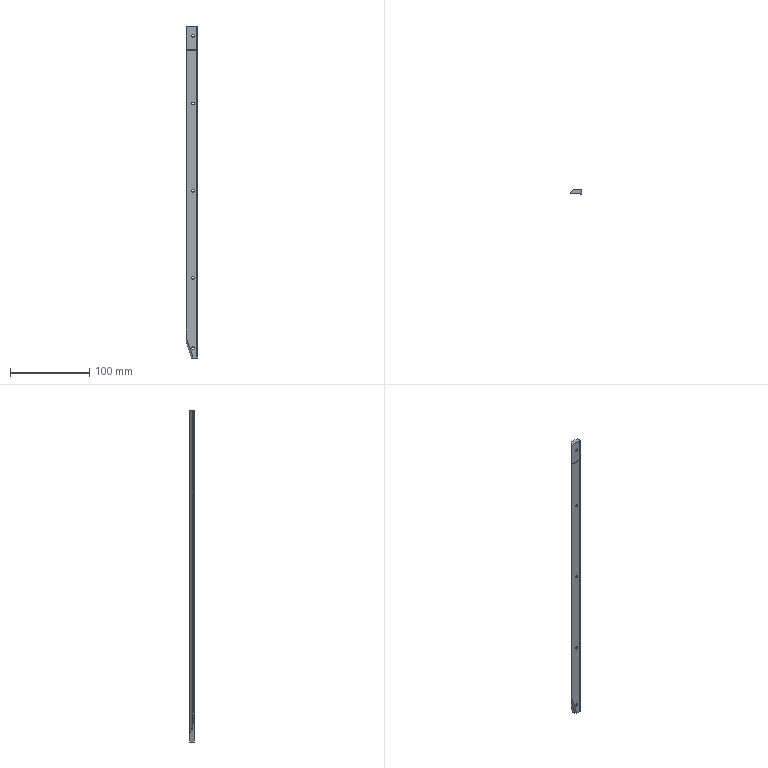Part | STEP file | 11-FG-B07511 | 1 solid | 43 faces | box 14.5 x 6 x 419 mm | volume 26571 mm3 | plane 22 | cylinder 21 | commonest cylinder face diameters 3.4 x10 6.5 x10 0.85 x1
STEP:
#1=CARTESIAN_POINT('',(8.5,1.6,403.25));
#2=VERTEX_POINT('',#1);
#3=CARTESIAN_POINT('',(8.5,1.6,409.75));
#4=VERTEX_POINT('',#3);
#5=CARTESIAN_POINT('',(8.5,1.6,406.5));
#6=DIRECTION('',(0.,1.,0.));
#7=DIRECTION('',(0.,0.,1.));
#8=AXIS2_PLACEMENT_3D('',#5,#6,#7);
#9=CIRCLE('',#8,3.25);
#10=EDGE_CURVE('',#2,#4,#9,.T.);
#11=ORIENTED_EDGE('',*,*,#10,.F.);
#12=CARTESIAN_POINT('',(8.5,5.,403.25));
#13=VERTEX_POINT('',#12);
#14=CARTESIAN_POINT('',(8.5,5.,403.25));
#15=DIRECTION('',(0.,1.,0.));
#16=VECTOR('',#15,1000.);
#17=LINE('',#14,#16);
#18=EDGE_CURVE('',#2,#13,#17,.T.);
#19=ORIENTED_EDGE('',*,*,#18,.T.);
#20=CARTESIAN_POINT('',(8.5,5.,409.75));
#21=VERTEX_POINT('',#20);
#22=CARTESIAN_POINT('',(8.5,5.,406.5));
#23=DIRECTION('',(0.,1.,0.));
#24=DIRECTION('',(0.,0.,1.));
#25=AXIS2_PLACEMENT_3D('',#22,#23,#24);
#26=CIRCLE('',#25,3.25);
#27=EDGE_CURVE('',#13,#21,#26,.T.);
#28=ORIENTED_EDGE('',*,*,#27,.T.);
#29=CARTESIAN_POINT('',(8.5,5.,409.75));
#30=DIRECTION('',(0.,1.,0.));
#31=VECTOR('',#30,1000.);
#32=LINE('',#29,#31);
#33=EDGE_CURVE('',#4,#21,#32,.T.);
#34=ORIENTED_EDGE('',*,*,#33,.F.);
#35=EDGE_LOOP('',(#11,#19,#28,#34));
#36=FACE_OUTER_BOUND('',#35,.T.);
#37=CARTESIAN_POINT('',(8.5,5.,406.5));
#38=DIRECTION('',(0.,1.,0.));
#39=DIRECTION('',(0.,0.,1.));
#40=AXIS2_PLACEMENT_3D('',#37,#38,#39);
#41=CYLINDRICAL_SURFACE('',#40,3.25);
#42=ADVANCED_FACE('',(#36),#41,.F.);
#43=CARTESIAN_POINT('',(8.5,0.,404.8));
#44=VERTEX_POINT('',#43);
#45=CARTESIAN_POINT('',(8.5,0.,408.2));
#46=VERTEX_POINT('',#45);
#47=CARTESIAN_POINT('',(8.5,0.,406.5));
#48=DIRECTION('',(0.,1.,0.));
#49=DIRECTION('',(0.,0.,1.));
#50=AXIS2_PLACEMENT_3D('',#47,#48,#49);
#51=CIRCLE('',#50,1.7);
#52=EDGE_CURVE('',#44,#46,#51,.T.);
#53=ORIENTED_EDGE('',*,*,#52,.F.);
#54=CARTESIAN_POINT('',(8.5,1.6,404.8));
#55=VERTEX_POINT('',#54);
#56=CARTESIAN_POINT('',(8.5,5.,404.8));
#57=DIRECTION('',(0.,1.,0.));
#58=VECTOR('',#57,1000.);
#59=LINE('',#56,#58);
#60=EDGE_CURVE('',#44,#55,#59,.T.);
#61=ORIENTED_EDGE('',*,*,#60,.T.);
#62=CARTESIAN_POINT('',(8.5,1.6,408.2));
#63=VERTEX_POINT('',#62);
#64=CARTESIAN_POINT('',(8.5,1.6,406.5));
#65=DIRECTION('',(0.,1.,0.));
#66=DIRECTION('',(0.,0.,1.));
#67=AXIS2_PLACEMENT_3D('',#64,#65,#66);
#68=CIRCLE('',#67,1.7);
#69=EDGE_CURVE('',#55,#63,#68,.T.);
#70=ORIENTED_EDGE('',*,*,#69,.T.);
#71=CARTESIAN_POINT('',(8.5,5.,408.2));
#72=DIRECTION('',(0.,1.,0.));
#73=VECTOR('',#72,1000.);
#74=LINE('',#71,#73);
#75=EDGE_CURVE('',#46,#63,#74,.T.);
#76=ORIENTED_EDGE('',*,*,#75,.F.);
#77=EDGE_LOOP('',(#53,#61,#70,#76));
#78=FACE_OUTER_BOUND('',#77,.T.);
#79=CARTESIAN_POINT('',(8.5,5.,406.5));
#80=DIRECTION('',(0.,1.,0.));
#81=DIRECTION('',(0.,0.,1.));
#82=AXIS2_PLACEMENT_3D('',#79,#80,#81);
#83=CYLINDRICAL_SURFACE('',#82,1.7);
#84=ADVANCED_FACE('',(#78),#83,.F.);
#85=CARTESIAN_POINT('',(8.5,1.6,317.75));
#86=VERTEX_POINT('',#85);
#87=CARTESIAN_POINT('',(8.5,1.6,324.25));
#88=VERTEX_POINT('',#87);
#89=CARTESIAN_POINT('',(8.5,1.6,321.));
#90=DIRECTION('',(0.,1.,0.));
#91=DIRECTION('',(0.,0.,1.));
#92=AXIS2_PLACEMENT_3D('',#89,#90,#91);
#93=CIRCLE('',#92,3.25);
#94=EDGE_CURVE('',#86,#88,#93,.T.);
#95=ORIENTED_EDGE('',*,*,#94,.F.);
#96=CARTESIAN_POINT('',(8.5,5.,317.75));
#97=VERTEX_POINT('',#96);
#98=CARTESIAN_POINT('',(8.5,5.,317.75));
#99=DIRECTION('',(0.,1.,0.));
#100=VECTOR('',#99,1000.);
#101=LINE('',#98,#100);
#102=EDGE_CURVE('',#86,#97,#101,.T.);
#103=ORIENTED_EDGE('',*,*,#102,.T.);
#104=CARTESIAN_POINT('',(8.5,5.,324.25));
#105=VERTEX_POINT('',#104);
#106=CARTESIAN_POINT('',(8.5,5.,321.));
#107=DIRECTION('',(0.,1.,0.));
#108=DIRECTION('',(0.,0.,1.));
#109=AXIS2_PLACEMENT_3D('',#106,#107,#108);
#110=CIRCLE('',#109,3.25);
#111=EDGE_CURVE('',#97,#105,#110,.T.);
#112=ORIENTED_EDGE('',*,*,#111,.T.);
#113=CARTESIAN_POINT('',(8.5,5.,324.25));
#114=DIRECTION('',(0.,1.,0.));
#115=VECTOR('',#114,1000.);
#116=LINE('',#113,#115);
#117=EDGE_CURVE('',#88,#105,#116,.T.);
#118=ORIENTED_EDGE('',*,*,#117,.F.);
#119=EDGE_LOOP('',(#95,#103,#112,#118));
#120=FACE_OUTER_BOUND('',#119,.T.);
#121=CARTESIAN_POINT('',(8.5,5.,321.));
#122=DIRECTION('',(0.,1.,0.));
#123=DIRECTION('',(0.,0.,1.));
#124=AXIS2_PLACEMENT_3D('',#121,#122,#123);
#125=CYLINDRICAL_SURFACE('',#124,3.25);
#126=ADVANCED_FACE('',(#120),#125,.F.);
#127=CARTESIAN_POINT('',(8.5,0.,319.3));
#128=VERTEX_POINT('',#127);
#129=CARTESIAN_POINT('',(8.5,0.,322.7));
#130=VERTEX_POINT('',#129);
#131=CARTESIAN_POINT('',(8.5,0.,321.));
#132=DIRECTION('',(0.,1.,0.));
#133=DIRECTION('',(0.,0.,1.));
#134=AXIS2_PLACEMENT_3D('',#131,#132,#133);
#135=CIRCLE('',#134,1.7);
#136=EDGE_CURVE('',#128,#130,#135,.T.);
#137=ORIENTED_EDGE('',*,*,#136,.F.);
#138=CARTESIAN_POINT('',(8.5,1.6,319.3));
#139=VERTEX_POINT('',#138);
#140=CARTESIAN_POINT('',(8.5,5.,319.3));
#141=DIRECTION('',(0.,1.,0.));
#142=VECTOR('',#141,1000.);
#143=LINE('',#140,#142);
#144=EDGE_CURVE('',#128,#139,#143,.T.);
#145=ORIENTED_EDGE('',*,*,#144,.T.);
#146=CARTESIAN_POINT('',(8.5,1.6,322.7));
#147=VERTEX_POINT('',#146);
#148=CARTESIAN_POINT('',(8.5,1.6,321.));
#149=DIRECTION('',(0.,1.,0.));
#150=DIRECTION('',(0.,0.,1.));
#151=AXIS2_PLACEMENT_3D('',#148,#149,#150);
#152=CIRCLE('',#151,1.7);
#153=EDGE_CURVE('',#139,#147,#152,.T.);
#154=ORIENTED_EDGE('',*,*,#153,.T.);
#155=CARTESIAN_POINT('',(8.5,5.,322.7));
#156=DIRECTION('',(0.,1.,0.));
#157=VECTOR('',#156,1000.);
#158=LINE('',#155,#157);
#159=EDGE_CURVE('',#130,#147,#158,.T.);
#160=ORIENTED_EDGE('',*,*,#159,.F.);
#161=EDGE_LOOP('',(#137,#145,#154,#160));
#162=FACE_OUTER_BOUND('',#161,.T.);
#163=CARTESIAN_POINT('',(8.5,5.,321.));
#164=DIRECTION('',(0.,1.,0.));
#165=DIRECTION('',(0.,0.,1.));
#166=AXIS2_PLACEMENT_3D('',#163,#164,#165);
#167=CYLINDRICAL_SURFACE('',#166,1.7);
#168=ADVANCED_FACE('',(#162),#167,.F.);
#169=CARTESIAN_POINT('',(8.5,1.6,207.75));
#170=VERTEX_POINT('',#169);
#171=CARTESIAN_POINT('',(8.5,1.6,214.25));
#172=VERTEX_POINT('',#171);
#173=CARTESIAN_POINT('',(8.5,1.6,211.));
#174=DIRECTION('',(0.,1.,0.));
#175=DIRECTION('',(0.,0.,1.));
#176=AXIS2_PLACEMENT_3D('',#173,#174,#175);
#177=CIRCLE('',#176,3.25);
#178=EDGE_CURVE('',#170,#172,#177,.T.);
#179=ORIENTED_EDGE('',*,*,#178,.F.);
#180=CARTESIAN_POINT('',(8.5,5.,207.75));
#181=VERTEX_POINT('',#180);
#182=CARTESIAN_POINT('',(8.5,5.,207.75));
#183=DIRECTION('',(0.,1.,0.));
#184=VECTOR('',#183,1000.);
#185=LINE('',#182,#184);
#186=EDGE_CURVE('',#170,#181,#185,.T.);
#187=ORIENTED_EDGE('',*,*,#186,.T.);
#188=CARTESIAN_POINT('',(8.5,5.,214.25));
#189=VERTEX_POINT('',#188);
#190=CARTESIAN_POINT('',(8.5,5.,211.));
#191=DIRECTION('',(0.,1.,0.));
#192=DIRECTION('',(0.,0.,1.));
#193=AXIS2_PLACEMENT_3D('',#190,#191,#192);
#194=CIRCLE('',#193,3.25);
#195=EDGE_CURVE('',#181,#189,#194,.T.);
#196=ORIENTED_EDGE('',*,*,#195,.T.);
#197=CARTESIAN_POINT('',(8.5,5.,214.25));
#198=DIRECTION('',(0.,1.,0.));
#199=VECTOR('',#198,1000.);
#200=LINE('',#197,#199);
#201=EDGE_CURVE('',#172,#189,#200,.T.);
#202=ORIENTED_EDGE('',*,*,#201,.F.);
#203=EDGE_LOOP('',(#179,#187,#196,#202));
#204=FACE_OUTER_BOUND('',#203,.T.);
#205=CARTESIAN_POINT('',(8.5,5.,211.));
#206=DIRECTION('',(0.,1.,0.));
#207=DIRECTION('',(0.,0.,1.));
#208=AXIS2_PLACEMENT_3D('',#205,#206,#207);
#209=CYLINDRICAL_SURFACE('',#208,3.25);
#210=ADVANCED_FACE('',(#204),#209,.F.);
#211=CARTESIAN_POINT('',(8.5,0.,209.3));
#212=VERTEX_POINT('',#211);
#213=CARTESIAN_POINT('',(8.5,0.,212.7));
#214=VERTEX_POINT('',#213);
#215=CARTESIAN_POINT('',(8.5,0.,211.));
#216=DIRECTION('',(0.,1.,0.));
#217=DIRECTION('',(0.,0.,1.));
#218=AXIS2_PLACEMENT_3D('',#215,#216,#217);
#219=CIRCLE('',#218,1.7);
#220=EDGE_CURVE('',#212,#214,#219,.T.);
#221=ORIENTED_EDGE('',*,*,#220,.F.);
#222=CARTESIAN_POINT('',(8.5,1.6,209.3));
#223=VERTEX_POINT('',#222);
#224=CARTESIAN_POINT('',(8.5,5.,209.3));
#225=DIRECTION('',(0.,1.,0.));
#226=VECTOR('',#225,1000.);
#227=LINE('',#224,#226);
#228=EDGE_CURVE('',#212,#223,#227,.T.);
#229=ORIENTED_EDGE('',*,*,#228,.T.);
#230=CARTESIAN_POINT('',(8.5,1.6,212.7));
#231=VERTEX_POINT('',#230);
#232=CARTESIAN_POINT('',(8.5,1.6,211.));
#233=DIRECTION('',(0.,1.,0.));
#234=DIRECTION('',(0.,0.,1.));
#235=AXIS2_PLACEMENT_3D('',#232,#233,#234);
#236=CIRCLE('',#235,1.7);
#237=EDGE_CURVE('',#223,#231,#236,.T.);
#238=ORIENTED_EDGE('',*,*,#237,.T.);
#239=CARTESIAN_POINT('',(8.5,5.,212.7));
#240=DIRECTION('',(0.,1.,0.));
#241=VECTOR('',#240,1000.);
#242=LINE('',#239,#241);
#243=EDGE_CURVE('',#214,#231,#242,.T.);
#244=ORIENTED_EDGE('',*,*,#243,.F.);
#245=EDGE_LOOP('',(#221,#229,#238,#244));
#246=FACE_OUTER_BOUND('',#245,.T.);
#247=CARTESIAN_POINT('',(8.5,5.,211.));
#248=DIRECTION('',(0.,1.,0.));
#249=DIRECTION('',(0.,0.,1.));
#250=AXIS2_PLACEMENT_3D('',#247,#248,#249);
#251=CYLINDRICAL_SURFACE('',#250,1.7);
#252=ADVANCED_FACE('',(#246),#251,.F.);
#253=CARTESIAN_POINT('',(8.5,1.6,97.75));
#254=VERTEX_POINT('',#253);
#255=CARTESIAN_POINT('',(8.5,1.6,104.25));
#256=VERTEX_POINT('',#255);
#257=CARTESIAN_POINT('',(8.5,1.6,101.));
#258=DIRECTION('',(0.,1.,0.));
#259=DIRECTION('',(0.,0.,1.));
#260=AXIS2_PLACEMENT_3D('',#257,#258,#259);
#261=CIRCLE('',#260,3.25);
#262=EDGE_CURVE('',#254,#256,#261,.T.);
#263=ORIENTED_EDGE('',*,*,#262,.F.);
#264=CARTESIAN_POINT('',(8.5,5.,97.75));
#265=VERTEX_POINT('',#264);
#266=CARTESIAN_POINT('',(8.5,5.,97.75));
#267=DIRECTION('',(0.,1.,0.));
#268=VECTOR('',#267,1000.);
#269=LINE('',#266,#268);
#270=EDGE_CURVE('',#254,#265,#269,.T.);
#271=ORIENTED_EDGE('',*,*,#270,.T.);
#272=CARTESIAN_POINT('',(8.5,5.,104.25));
#273=VERTEX_POINT('',#272);
#274=CARTESIAN_POINT('',(8.5,5.,101.));
#275=DIRECTION('',(0.,1.,0.));
#276=DIRECTION('',(0.,0.,1.));
#277=AXIS2_PLACEMENT_3D('',#274,#275,#276);
#278=CIRCLE('',#277,3.25);
#279=EDGE_CURVE('',#265,#273,#278,.T.);
#280=ORIENTED_EDGE('',*,*,#279,.T.);
#281=CARTESIAN_POINT('',(8.5,5.,104.25));
#282=DIRECTION('',(0.,1.,0.));
#283=VECTOR('',#282,1000.);
#284=LINE('',#281,#283);
#285=EDGE_CURVE('',#256,#273,#284,.T.);
#286=ORIENTED_EDGE('',*,*,#285,.F.);
#287=EDGE_LOOP('',(#263,#271,#280,#286));
#288=FACE_OUTER_BOUND('',#287,.T.);
#289=CARTESIAN_POINT('',(8.5,5.,101.));
#290=DIRECTION('',(0.,1.,0.));
#291=DIRECTION('',(0.,0.,1.));
#292=AXIS2_PLACEMENT_3D('',#289,#290,#291);
#293=CYLINDRICAL_SURFACE('',#292,3.25);
#294=ADVANCED_FACE('',(#288),#293,.F.);
#295=CARTESIAN_POINT('',(8.5,0.,99.3));
#296=VERTEX_POINT('',#295);
#297=CARTESIAN_POINT('',(8.5,0.,102.7));
#298=VERTEX_POINT('',#297);
#299=CARTESIAN_POINT('',(8.5,0.,101.));
#300=DIRECTION('',(0.,1.,0.));
#301=DIRECTION('',(0.,0.,1.));
#302=AXIS2_PLACEMENT_3D('',#299,#300,#301);
#303=CIRCLE('',#302,1.7);
#304=EDGE_CURVE('',#296,#298,#303,.T.);
#305=ORIENTED_EDGE('',*,*,#304,.F.);
#306=CARTESIAN_POINT('',(8.5,1.6,99.3));
#307=VERTEX_POINT('',#306);
#308=CARTESIAN_POINT('',(8.5,5.,99.3));
#309=DIRECTION('',(0.,1.,0.));
#310=VECTOR('',#309,1000.);
#311=LINE('',#308,#310);
#312=EDGE_CURVE('',#296,#307,#311,.T.);
#313=ORIENTED_EDGE('',*,*,#312,.T.);
#314=CARTESIAN_POINT('',(8.5,1.6,102.7));
#315=VERTEX_POINT('',#314);
#316=CARTESIAN_POINT('',(8.5,1.6,101.));
#317=DIRECTION('',(0.,1.,0.));
#318=DIRECTION('',(0.,0.,1.));
#319=AXIS2_PLACEMENT_3D('',#316,#317,#318);
#320=CIRCLE('',#319,1.7);
#321=EDGE_CURVE('',#307,#315,#320,.T.);
#322=ORIENTED_EDGE('',*,*,#321,.T.);
#323=CARTESIAN_POINT('',(8.5,5.,102.7));
#324=DIRECTION('',(0.,1.,0.));
#325=VECTOR('',#324,1000.);
#326=LINE('',#323,#325);
#327=EDGE_CURVE('',#298,#315,#326,.T.);
#328=ORIENTED_EDGE('',*,*,#327,.F.);
#329=EDGE_LOOP('',(#305,#313,#322,#328));
#330=FACE_OUTER_BOUND('',#329,.T.);
#331=CARTESIAN_POINT('',(8.5,5.,101.));
#332=DIRECTION('',(0.,1.,0.));
#333=DIRECTION('',(0.,0.,1.));
#334=AXIS2_PLACEMENT_3D('',#331,#332,#333);
#335=CYLINDRICAL_SURFACE('',#334,1.7);
#336=ADVANCED_FACE('',(#330),#335,.F.);
#337=CARTESIAN_POINT('',(8.5,1.6,9.25));
#338=VERTEX_POINT('',#337);
#339=CARTESIAN_POINT('',(8.5,1.6,15.75));
#340=VERTEX_POINT('',#339);
#341=CARTESIAN_POINT('',(8.5,1.6,12.5));
#342=DIRECTION('',(0.,1.,0.));
#343=DIRECTION('',(0.,0.,1.));
#344=AXIS2_PLACEMENT_3D('',#341,#342,#343);
#345=CIRCLE('',#344,3.25);
#346=EDGE_CURVE('',#338,#340,#345,.T.);
#347=ORIENTED_EDGE('',*,*,#346,.F.);
#348=CARTESIAN_POINT('',(8.5,5.,9.25));
#349=VERTEX_POINT('',#348);
#350=CARTESIAN_POINT('',(8.5,5.,9.25));
#351=DIRECTION('',(0.,1.,0.));
#352=VECTOR('',#351,1000.);
#353=LINE('',#350,#352);
#354=EDGE_CURVE('',#338,#349,#353,.T.);
#355=ORIENTED_EDGE('',*,*,#354,.T.);
#356=CARTESIAN_POINT('',(8.5,5.,15.75));
#357=VERTEX_POINT('',#356);
#358=CARTESIAN_POINT('',(8.5,5.,12.5));
#359=DIRECTION('',(0.,1.,0.));
#360=DIRECTION('',(0.,0.,1.));
#361=AXIS2_PLACEMENT_3D('',#358,#359,#360);
#362=CIRCLE('',#361,3.25);
#363=EDGE_CURVE('',#349,#357,#362,.T.);
#364=ORIENTED_EDGE('',*,*,#363,.T.);
#365=CARTESIAN_POINT('',(8.5,5.,15.75));
#366=DIRECTION('',(0.,1.,0.));
#367=VECTOR('',#366,1000.);
#368=LINE('',#365,#367);
#369=EDGE_CURVE('',#340,#357,#368,.T.);
#370=ORIENTED_EDGE('',*,*,#369,.F.);
#371=EDGE_LOOP('',(#347,#355,#364,#370));
#372=FACE_OUTER_BOUND('',#371,.T.);
#373=CARTESIAN_POINT('',(8.5,5.,12.5));
#374=DIRECTION('',(0.,1.,0.));
#375=DIRECTION('',(0.,0.,1.));
#376=AXIS2_PLACEMENT_3D('',#373,#374,#375);
#377=CYLINDRICAL_SURFACE('',#376,3.25);
#378=ADVANCED_FACE('',(#372),#377,.F.);
#379=CARTESIAN_POINT('',(8.5,0.,10.8));
#380=VERTEX_POINT('',#379);
#381=CARTESIAN_POINT('',(8.5,0.,14.2));
#382=VERTEX_POINT('',#381);
#383=CARTESIAN_POINT('',(8.5,0.,12.5));
#384=DIRECTION('',(0.,1.,0.));
#385=DIRECTION('',(0.,0.,1.));
#386=AXIS2_PLACEMENT_3D('',#383,#384,#385);
#387=CIRCLE('',#386,1.7);
#388=EDGE_CURVE('',#380,#382,#387,.T.);
#389=ORIENTED_EDGE('',*,*,#388,.F.);
#390=CARTESIAN_POINT('',(8.5,1.6,10.8));
#391=VERTEX_POINT('',#390);
#392=CARTESIAN_POINT('',(8.5,5.,10.8));
#393=DIRECTION('',(0.,1.,0.));
#394=VECTOR('',#393,1000.);
#395=LINE('',#392,#394);
#396=EDGE_CURVE('',#380,#391,#395,.T.);
#397=ORIENTED_EDGE('',*,*,#396,.T.);
#398=CARTESIAN_POINT('',(8.5,1.6,14.2));
#399=VERTEX_POINT('',#398);
#400=CARTESIAN_POINT('',(8.5,1.6,12.5));
#401=DIRECTION('',(0.,1.,0.));
#402=DIRECTION('',(0.,0.,1.));
#403=AXIS2_PLACEMENT_3D('',#400,#401,#402);
#404=CIRCLE('',#403,1.7);
#405=EDGE_CURVE('',#391,#399,#404,.T.);
#406=ORIENTED_EDGE('',*,*,#405,.T.);
#407=CARTESIAN_POINT('',(8.5,5.,14.2));
#408=DIRECTION('',(0.,1.,0.));
#409=VECTOR('',#408,1000.);
#410=LINE('',#407,#409);
#411=EDGE_CURVE('',#382,#399,#410,.T.);
#412=ORIENTED_EDGE('',*,*,#411,.F.);
#413=EDGE_LOOP('',(#389,#397,#406,#412));
#414=FACE_OUTER_BOUND('',#413,.T.);
#415=CARTESIAN_POINT('',(8.5,5.,12.5));
#416=DIRECTION('',(0.,1.,0.));
#417=DIRECTION('',(0.,0.,1.));
#418=AXIS2_PLACEMENT_3D('',#415,#416,#417);
#419=CYLINDRICAL_SURFACE('',#418,1.7);
#420=ADVANCED_FACE('',(#414),#419,.F.);
#421=CARTESIAN_POINT('',(0.,1.,419.));
#422=VERTEX_POINT('',#421);
#423=CARTESIAN_POINT('',(0.,1.,389.144));
#424=VERTEX_POINT('',#423);
#425=CARTESIAN_POINT('',(0.,1.,419.));
#426=DIRECTION('',(0.,0.,-1.));
#427=VECTOR('',#426,1000.);
#428=LINE('',#425,#427);
#429=EDGE_CURVE('',#422,#424,#428,.T.);
#430=ORIENTED_EDGE('',*,*,#429,.T.);
#431=CARTESIAN_POINT('',(0.,0.6,389.425));
#432=VERTEX_POINT('',#431);
#433=CARTESIAN_POINT('',(0.,0.6,389.));
#434=DIRECTION('',(-1.,0.,0.));
#435=DIRECTION('',(0.,0.,1.));
#436=AXIS2_PLACEMENT_3D('',#433,#434,#435);
#437=CIRCLE('',#436,0.425);
#438=EDGE_CURVE('',#432,#424,#437,.T.);
#439=ORIENTED_EDGE('',*,*,#438,.F.);
#440=CARTESIAN_POINT('',(0.,0.,389.425));
#441=VERTEX_POINT('',#440);
#442=CARTESIAN_POINT('',(0.,0.6,389.425));
#443=DIRECTION('',(0.,1.,0.));
#444=VECTOR('',#443,1000.);
#445=LINE('',#442,#444);
#446=EDGE_CURVE('',#441,#432,#445,.T.);
#447=ORIENTED_EDGE('',*,*,#446,.F.);
#448=CARTESIAN_POINT('',(0.,0.,419.));
#449=VERTEX_POINT('',#448);
#450=CARTESIAN_POINT('',(0.,0.,419.));
#451=DIRECTION('',(0.,0.,-1.));
#452=VECTOR('',#451,1000.);
#453=LINE('',#450,#452);
#454=EDGE_CURVE('',#449,#441,#453,.T.);
#455=ORIENTED_EDGE('',*,*,#454,.F.);
#456=CARTESIAN_POINT('',(0.,0.,419.));
#457=DIRECTION('',(0.,-1.,0.));
#458=VECTOR('',#457,1000.);
#459=LINE('',#456,#458);
#460=EDGE_CURVE('',#422,#449,#459,.T.);
#461=ORIENTED_EDGE('',*,*,#460,.F.);
#462=EDGE_LOOP('',(#430,#439,#447,#455,#461));
#463=FACE_OUTER_BOUND('',#462,.T.);
#464=CARTESIAN_POINT('',(0.,0.,419.));
#465=DIRECTION('',(1.,0.,0.));
#466=DIRECTION('',(0.,1.,0.));
#467=AXIS2_PLACEMENT_3D('',#464,#465,#466);
#468=PLANE('',#467);
#469=ADVANCED_FACE('',(#463),#468,.F.);
#470=CARTESIAN_POINT('',(8.5,0.,406.5));
#471=DIRECTION('',(0.,1.,0.));
#472=DIRECTION('',(0.,0.,1.));
#473=AXIS2_PLACEMENT_3D('',#470,#471,#472);
#474=CIRCLE('',#473,1.7);
#475=EDGE_CURVE('',#46,#44,#474,.T.);
#476=ORIENTED_EDGE('',*,*,#475,.T.);
#477=ORIENTED_EDGE('',*,*,#52,.T.);
#478=EDGE_LOOP('',(#476,#477));
#479=FACE_BOUND('',#478,.T.);
#480=ORIENTED_EDGE('',*,*,#454,.T.);
#481=CARTESIAN_POINT('',(13.5,0.,389.425));
#482=VERTEX_POINT('',#481);
#483=CARTESIAN_POINT('',(13.5,0.,389.425));
#484=DIRECTION('',(-1.,0.,0.));
#485=VECTOR('',#484,1000.);
#486=LINE('',#483,#485);
#487=EDGE_CURVE('',#482,#441,#486,.T.);
#488=ORIENTED_EDGE('',*,*,#487,.F.);
#489=CARTESIAN_POINT('',(13.5,0.,419.));
#490=VERTEX_POINT('',#489);
#491=CARTESIAN_POINT('',(13.5,0.,419.));
#492=DIRECTION('',(0.,0.,-1.));
#493=VECTOR('',#492,1000.);
#494=LINE('',#491,#493);
#495=EDGE_CURVE('',#490,#482,#494,.T.);
#496=ORIENTED_EDGE('',*,*,#495,.F.);
#497=CARTESIAN_POINT('',(0.,0.,419.));
#498=DIRECTION('',(1.,0.,0.));
#499=VECTOR('',#498,1000.);
#500=LINE('',#497,#499);
#501=EDGE_CURVE('',#449,#490,#500,.T.);
#502=ORIENTED_EDGE('',*,*,#501,.F.);
#503=EDGE_LOOP('',(#480,#488,#496,#502));
#504=FACE_OUTER_BOUND('',#503,.T.);
#505=CARTESIAN_POINT('',(0.,0.,419.));
#506=DIRECTION('',(0.,1.,0.));
#507=DIRECTION('',(0.,0.,1.));
#508=AXIS2_PLACEMENT_3D('',#505,#506,#507);
#509=PLANE('',#508);
#510=ADVANCED_FACE('',(#479,#504),#509,.F.);
#511=CARTESIAN_POINT('',(0.,1.,388.856));
#512=VERTEX_POINT('',#511);
#513=CARTESIAN_POINT('',(0.,1.,20.867));
#514=VERTEX_POINT('',#513);
#515=CARTESIAN_POINT('',(0.,1.,419.));
#516=DIRECTION('',(0.,0.,-1.));
#517=VECTOR('',#516,1000.);
#518=LINE('',#515,#517);
#519=EDGE_CURVE('',#512,#514,#518,.T.);
#520=ORIENTED_EDGE('',*,*,#519,.T.);
#521=CARTESIAN_POINT('',(0.,0.,26.471));
#522=VERTEX_POINT('',#521);
#523=CARTESIAN_POINT('',(0.,-61.4,370.543));
#524=DIRECTION('',(0.,-0.1757,0.9844));
#525=VECTOR('',#524,1000.);
#526=LINE('',#523,#525);
#527=EDGE_CURVE('',#514,#522,#526,.T.);
#528=ORIENTED_EDGE('',*,*,#527,.T.);
#529=CARTESIAN_POINT('',(0.,0.,388.575));
#530=VERTEX_POINT('',#529);
#531=CARTESIAN_POINT('',(0.,0.,419.));
#532=DIRECTION('',(0.,0.,-1.));
#533=VECTOR('',#532,1000.);
#534=LINE('',#531,#533);
#535=EDGE_CURVE('',#530,#522,#534,.T.);
#536=ORIENTED_EDGE('',*,*,#535,.F.);
#537=CARTESIAN_POINT('',(0.,0.6,388.575));
#538=VERTEX_POINT('',#537);
#539=CARTESIAN_POINT('',(0.,0.6,388.575));
#540=DIRECTION('',(0.,-1.,0.));
#541=VECTOR('',#540,1000.);
#542=LINE('',#539,#541);
#543=EDGE_CURVE('',#538,#530,#542,.T.);
#544=ORIENTED_EDGE('',*,*,#543,.F.);
#545=CARTESIAN_POINT('',(0.,0.6,389.));
#546=DIRECTION('',(-1.,0.,0.));
#547=DIRECTION('',(0.,0.,1.));
#548=AXIS2_PLACEMENT_3D('',#545,#546,#547);
#549=CIRCLE('',#548,0.425);
#550=EDGE_CURVE('',#512,#538,#549,.T.);
#551=ORIENTED_EDGE('',*,*,#550,.F.);
#552=EDGE_LOOP('',(#520,#528,#536,#544,#551));
#553=FACE_OUTER_BOUND('',#552,.T.);
#554=CARTESIAN_POINT('',(0.,0.,419.));
#555=DIRECTION('',(1.,0.,0.));
#556=DIRECTION('',(0.,1.,0.));
#557=AXIS2_PLACEMENT_3D('',#554,#555,#556);
#558=PLANE('',#557);
#559=ADVANCED_FACE('',(#553),#558,.F.);
#560=CARTESIAN_POINT('',(8.5,0.,321.));
#561=DIRECTION('',(0.,1.,0.));
#562=DIRECTION('',(0.,0.,1.));
#563=AXIS2_PLACEMENT_3D('',#560,#561,#562);
#564=CIRCLE('',#563,1.7);
#565=EDGE_CURVE('',#130,#128,#564,.T.);
#566=ORIENTED_EDGE('',*,*,#565,.T.);
#567=ORIENTED_EDGE('',*,*,#136,.T.);
#568=EDGE_LOOP('',(#566,#567));
#569=FACE_BOUND('',#568,.T.);
#570=CARTESIAN_POINT('',(8.5,0.,211.));
#571=DIRECTION('',(0.,1.,0.));
#572=DIRECTION('',(0.,0.,1.));
#573=AXIS2_PLACEMENT_3D('',#570,#571,#572);
#574=CIRCLE('',#573,1.7);
#575=EDGE_CURVE('',#214,#212,#574,.T.);
#576=ORIENTED_EDGE('',*,*,#575,.T.);
#577=ORIENTED_EDGE('',*,*,#220,.T.);
#578=EDGE_LOOP('',(#576,#577));
#579=FACE_BOUND('',#578,.T.);
#580=CARTESIAN_POINT('',(8.5,0.,101.));
#581=DIRECTION('',(0.,1.,0.));
#582=DIRECTION('',(0.,0.,1.));
#583=AXIS2_PLACEMENT_3D('',#580,#581,#582);
#584=CIRCLE('',#583,1.7);
#585=EDGE_CURVE('',#298,#296,#584,.T.);
#586=ORIENTED_EDGE('',*,*,#585,.T.);
#587=ORIENTED_EDGE('',*,*,#304,.T.);
#588=EDGE_LOOP('',(#586,#587));
#589=FACE_BOUND('',#588,.T.);
#590=CARTESIAN_POINT('',(8.5,0.,12.5));
#591=DIRECTION('',(0.,1.,0.));
#592=DIRECTION('',(0.,0.,1.));
#593=AXIS2_PLACEMENT_3D('',#590,#591,#592);
#594=CIRCLE('',#593,1.7);
#595=EDGE_CURVE('',#382,#380,#594,.T.);
#596=ORIENTED_EDGE('',*,*,#595,.T.);
#597=ORIENTED_EDGE('',*,*,#388,.T.);
#598=EDGE_LOOP('',(#596,#597));
#599=FACE_BOUND('',#598,.T.);
#600=ORIENTED_EDGE('',*,*,#535,.T.);
#601=CARTESIAN_POINT('',(8.603,0.,0.));
#602=VERTEX_POINT('',#601);
#603=CARTESIAN_POINT('',(-115.385,0.,381.5));
#604=DIRECTION('',(0.3091,0.,-0.951));
#605=VECTOR('',#604,1000.);
#606=LINE('',#603,#605);
#607=EDGE_CURVE('',#522,#602,#606,.T.);
#608=ORIENTED_EDGE('',*,*,#607,.T.);
#609=CARTESIAN_POINT('',(13.5,0.,0.));
#610=VERTEX_POINT('',#609);
#611=CARTESIAN_POINT('',(0.,0.,0.));
#612=DIRECTION('',(1.,0.,0.));
#613=VECTOR('',#612,1000.);
#614=LINE('',#611,#613);
#615=EDGE_CURVE('',#602,#610,#614,.T.);
#616=ORIENTED_EDGE('',*,*,#615,.T.);
#617=CARTESIAN_POINT('',(13.5,0.,388.575));
#618=VERTEX_POINT('',#617);
#619=CARTESIAN_POINT('',(13.5,0.,419.));
#620=DIRECTION('',(0.,0.,-1.));
#621=VECTOR('',#620,1000.);
#622=LINE('',#619,#621);
#623=EDGE_CURVE('',#618,#610,#622,.T.);
#624=ORIENTED_EDGE('',*,*,#623,.F.);
#625=CARTESIAN_POINT('',(13.5,0.,388.575));
#626=DIRECTION('',(-1.,0.,0.));
#627=VECTOR('',#626,1000.);
#628=LINE('',#625,#627);
#629=EDGE_CURVE('',#618,#530,#628,.T.);
#630=ORIENTED_EDGE('',*,*,#629,.T.);
#631=EDGE_LOOP('',(#600,#608,#616,#624,#630));
#632=FACE_OUTER_BOUND('',#631,.T.);
#633=CARTESIAN_POINT('',(0.,0.,419.));
#634=DIRECTION('',(0.,1.,0.));
#635=DIRECTION('',(0.,0.,1.));
#636=AXIS2_PLACEMENT_3D('',#633,#634,#635);
#637=PLANE('',#636);
#638=ADVANCED_FACE('',(#569,#579,#589,#599,#632),#637,.F.);
#639=CARTESIAN_POINT('',(8.5,5.,406.5));
#640=DIRECTION('',(0.,1.,0.));
#641=DIRECTION('',(0.,0.,1.));
#642=AXIS2_PLACEMENT_3D('',#639,#640,#641);
#643=CIRCLE('',#642,3.25);
#644=EDGE_CURVE('',#21,#13,#643,.T.);
#645=ORIENTED_EDGE('',*,*,#644,.F.);
#646=ORIENTED_EDGE('',*,*,#27,.F.);
#647=EDGE_LOOP('',(#645,#646));
#648=FACE_BOUND('',#647,.T.);
#649=CARTESIAN_POINT('',(8.5,5.,321.));
#650=DIRECTION('',(0.,1.,0.));
#651=DIRECTION('',(0.,0.,1.));
#652=AXIS2_PLACEMENT_3D('',#649,#650,#651);
#653=CIRCLE('',#652,3.25);
#654=EDGE_CURVE('',#105,#97,#653,.T.);
#655=ORIENTED_EDGE('',*,*,#654,.F.);
#656=ORIENTED_EDGE('',*,*,#111,.F.);
#657=EDGE_LOOP('',(#655,#656));
#658=FACE_BOUND('',#657,.T.);
#659=CARTESIAN_POINT('',(8.5,5.,211.));
#660=DIRECTION('',(0.,1.,0.));
#661=DIRECTION('',(0.,0.,1.));
#662=AXIS2_PLACEMENT_3D('',#659,#660,#661);
#663=CIRCLE('',#662,3.25);
#664=EDGE_CURVE('',#189,#181,#663,.T.);
#665=ORIENTED_EDGE('',*,*,#664,.F.);
#666=ORIENTED_EDGE('',*,*,#195,.F.);
#667=EDGE_LOOP('',(#665,#666));
#668=FACE_BOUND('',#667,.T.);
#669=CARTESIAN_POINT('',(8.5,5.,101.));
#670=DIRECTION('',(0.,1.,0.));
#671=DIRECTION('',(0.,0.,1.));
#672=AXIS2_PLACEMENT_3D('',#669,#670,#671);
#673=CIRCLE('',#672,3.25);
#674=EDGE_CURVE('',#273,#265,#673,.T.);
#675=ORIENTED_EDGE('',*,*,#674,.F.);
#676=ORIENTED_EDGE('',*,*,#279,.F.);
#677=EDGE_LOOP('',(#675,#676));
#678=FACE_BOUND('',#677,.T.);
#679=CARTESIAN_POINT('',(8.5,5.,12.5));
#680=DIRECTION('',(0.,1.,0.));
#681=DIRECTION('',(0.,0.,1.));
#682=AXIS2_PLACEMENT_3D('',#679,#680,#681);
#683=CIRCLE('',#682,3.25);
#684=EDGE_CURVE('',#357,#349,#683,.T.);
#685=ORIENTED_EDGE('',*,*,#684,.F.);
#686=ORIENTED_EDGE('',*,*,#363,.F.);
#687=EDGE_LOOP('',(#685,#686));
#688=FACE_BOUND('',#687,.T.);
#689=CARTESIAN_POINT('',(14.5,5.,0.));
#690=VERTEX_POINT('',#689);
#691=CARTESIAN_POINT('',(6.5,5.,0.));
#692=VERTEX_POINT('',#691);
#693=CARTESIAN_POINT('',(0.,5.,0.));
#694=DIRECTION('',(-1.,0.,0.));
#695=VECTOR('',#694,1000.);
#696=LINE('',#693,#695);
#697=EDGE_CURVE('',#690,#692,#696,.T.);
#698=ORIENTED_EDGE('',*,*,#697,.T.);
#699=CARTESIAN_POINT('',(4.,5.,7.692));
#700=VERTEX_POINT('',#699);
#701=CARTESIAN_POINT('',(6.5,5.,0.));
#702=DIRECTION('',(0.3091,0.,-0.951));
#703=VECTOR('',#702,1000.);
#704=LINE('',#701,#703);
#705=EDGE_CURVE('',#700,#692,#704,.T.);
#706=ORIENTED_EDGE('',*,*,#705,.F.);
#707=CARTESIAN_POINT('',(4.,5.,419.));
#708=VERTEX_POINT('',#707);
#709=CARTESIAN_POINT('',(4.,5.,419.));
#710=DIRECTION('',(0.,0.,1.));
#711=VECTOR('',#710,1000.);
#712=LINE('',#709,#711);
#713=EDGE_CURVE('',#700,#708,#712,.T.);
#714=ORIENTED_EDGE('',*,*,#713,.T.);
#715=CARTESIAN_POINT('',(14.5,5.,419.));
#716=VERTEX_POINT('',#715);
#717=CARTESIAN_POINT('',(0.,5.,419.));
#718=DIRECTION('',(-1.,0.,0.));
#719=VECTOR('',#718,1000.);
#720=LINE('',#717,#719);
#721=EDGE_CURVE('',#716,#708,#720,.T.);
#722=ORIENTED_EDGE('',*,*,#721,.F.);
#723=CARTESIAN_POINT('',(14.5,5.,419.));
#724=DIRECTION('',(0.,0.,1.));
#725=VECTOR('',#724,1000.);
#726=LINE('',#723,#725);
#727=EDGE_CURVE('',#690,#716,#726,.T.);
#728=ORIENTED_EDGE('',*,*,#727,.F.);
#729=EDGE_LOOP('',(#698,#706,#714,#722,#728));
#730=FACE_OUTER_BOUND('',#729,.T.);
#731=CARTESIAN_POINT('',(0.,5.,419.));
#732=DIRECTION('',(0.,-1.,0.));
#733=DIRECTION('',(0.,0.,-1.));
#734=AXIS2_PLACEMENT_3D('',#731,#732,#733);
#735=PLANE('',#734);
#736=ADVANCED_FACE('',(#648,#658,#668,#678,#688,#730),#735,.F.);
#737=ORIENTED_EDGE('',*,*,#721,.T.);
#738=CARTESIAN_POINT('',(0.,1.,419.));
#739=DIRECTION('',(-0.7071,-0.7071,0.));
#740=VECTOR('',#739,1000.);
#741=LINE('',#738,#740);
#742=EDGE_CURVE('',#708,#422,#741,.T.);
#743=ORIENTED_EDGE('',*,*,#742,.T.);
#744=ORIENTED_EDGE('',*,*,#460,.T.);
#745=ORIENTED_EDGE('',*,*,#501,.T.);
#746=CARTESIAN_POINT('',(13.5,-1.,419.));
#747=VERTEX_POINT('',#746);
#748=CARTESIAN_POINT('',(13.5,5.,419.));
#749=DIRECTION('',(0.,-1.,0.));
#750=VECTOR('',#749,1000.);
#751=LINE('',#748,#750);
#752=EDGE_CURVE('',#490,#747,#751,.T.);
#753=ORIENTED_EDGE('',*,*,#752,.T.);
#754=CARTESIAN_POINT('',(14.5,-1.,419.));
#755=VERTEX_POINT('',#754);
#756=CARTESIAN_POINT('',(14.5,-1.,419.));
#757=DIRECTION('',(-1.,0.,0.));
#758=VECTOR('',#757,1000.);
#759=LINE('',#756,#758);
#760=EDGE_CURVE('',#755,#747,#759,.T.);
#761=ORIENTED_EDGE('',*,*,#760,.F.);
#762=CARTESIAN_POINT('',(14.5,5.,419.));
#763=DIRECTION('',(0.,-1.,0.));
#764=VECTOR('',#763,1000.);
#765=LINE('',#762,#764);
#766=EDGE_CURVE('',#716,#755,#765,.T.);
#767=ORIENTED_EDGE('',*,*,#766,.F.);
#768=EDGE_LOOP('',(#737,#743,#744,#745,#753,#761,#767));
#769=FACE_OUTER_BOUND('',#768,.T.);
#770=CARTESIAN_POINT('',(0.,5.,419.));
#771=DIRECTION('',(0.,0.,-1.));
#772=DIRECTION('',(-1.,0.,0.));
#773=AXIS2_PLACEMENT_3D('',#770,#771,#772);
#774=PLANE('',#773);
#775=ADVANCED_FACE('',(#769),#774,.F.);
#776=ORIENTED_EDGE('',*,*,#615,.F.);
#777=CARTESIAN_POINT('',(6.5,1.155,0.));
#778=VERTEX_POINT('',#777);
#779=CARTESIAN_POINT('',(-0.1166,4.788,0.));
#780=DIRECTION('',(-0.8766,0.4813,0.));
#781=VECTOR('',#780,1000.);
#782=LINE('',#779,#781);
#783=EDGE_CURVE('',#602,#778,#782,.T.);
#784=ORIENTED_EDGE('',*,*,#783,.T.);
#785=CARTESIAN_POINT('',(6.5,-5.,0.));
#786=DIRECTION('',(0.,1.,0.));
#787=VECTOR('',#786,1000.);
#788=LINE('',#785,#787);
#789=EDGE_CURVE('',#778,#692,#788,.T.);
#790=ORIENTED_EDGE('',*,*,#789,.T.);
#791=ORIENTED_EDGE('',*,*,#697,.F.);
#792=CARTESIAN_POINT('',(14.5,-1.,0.));
#793=VERTEX_POINT('',#792);
#794=CARTESIAN_POINT('',(14.5,5.,0.));
#795=DIRECTION('',(0.,1.,0.));
#796=VECTOR('',#795,1000.);
#797=LINE('',#794,#796);
#798=EDGE_CURVE('',#793,#690,#797,.T.);
#799=ORIENTED_EDGE('',*,*,#798,.F.);
#800=CARTESIAN_POINT('',(13.5,-1.,0.));
#801=VERTEX_POINT('',#800);
#802=CARTESIAN_POINT('',(14.5,-1.,0.));
#803=DIRECTION('',(-1.,0.,0.));
#804=VECTOR('',#803,1000.);
#805=LINE('',#802,#804);
#806=EDGE_CURVE('',#793,#801,#805,.T.);
#807=ORIENTED_EDGE('',*,*,#806,.T.);
#808=CARTESIAN_POINT('',(13.5,5.,0.));
#809=DIRECTION('',(0.,1.,0.));
#810=VECTOR('',#809,1000.);
#811=LINE('',#808,#810);
#812=EDGE_CURVE('',#801,#610,#811,.T.);
#813=ORIENTED_EDGE('',*,*,#812,.T.);
#814=EDGE_LOOP('',(#776,#784,#790,#791,#799,#807,#813));
#815=FACE_OUTER_BOUND('',#814,.T.);
#816=CARTESIAN_POINT('',(0.,5.,0.));
#817=DIRECTION('',(0.,0.,-1.));
#818=DIRECTION('',(-1.,0.,0.));
#819=AXIS2_PLACEMENT_3D('',#816,#817,#818);
#820=PLANE('',#819);
#821=ADVANCED_FACE('',(#815),#820,.T.);
#822=CARTESIAN_POINT('',(0.1547,1.155,19.524));
#823=VERTEX_POINT('',#822);
#824=CARTESIAN_POINT('',(-107.059,-106.059,349.412));
#825=DIRECTION('',(0.2953,0.2953,-0.9086));
#826=VECTOR('',#825,1000.);
#827=LINE('',#824,#826);
#828=EDGE_CURVE('',#823,#700,#827,.T.);
#829=ORIENTED_EDGE('',*,*,#828,.F.);
#830=CARTESIAN_POINT('',(-44.678,-43.678,408.706));
#831=DIRECTION('',(-0.1137,-0.1137,0.987));
#832=VECTOR('',#831,1000.);
#833=LINE('',#830,#832);
#834=EDGE_CURVE('',#823,#514,#833,.T.);
#835=ORIENTED_EDGE('',*,*,#834,.T.);
#836=ORIENTED_EDGE('',*,*,#519,.F.);
#837=CARTESIAN_POINT('',(0.,1.,389.144));
#838=CARTESIAN_POINT('',(0.03367,1.034,389.05));
#839=CARTESIAN_POINT('',(0.03367,1.034,388.95));
#840=CARTESIAN_POINT('',(0.,1.,388.856));
#841=(BOUNDED_CURVE()B_SPLINE_CURVE(3,(#837,#838,#839,#840),.UNSPECIFIED.,.F.,.F.)B_SPLINE_CURVE_WITH_KNOTS((4,4),(2.797,3.486),.UNSPECIFIED.)CURVE()GEOMETRIC_REPRESENTATION_ITEM()RATIONAL_B_SPLINE_CURVE((1.,0.9608,0.9608,1.))REPRESENTATION_ITEM(''));
#842=EDGE_CURVE('',#424,#512,#841,.T.);
#843=ORIENTED_EDGE('',*,*,#842,.F.);
#844=ORIENTED_EDGE('',*,*,#429,.F.);
#845=ORIENTED_EDGE('',*,*,#742,.F.);
#846=ORIENTED_EDGE('',*,*,#713,.F.);
#847=EDGE_LOOP('',(#829,#835,#836,#843,#844,#845,#846));
#848=FACE_OUTER_BOUND('',#847,.T.);
#849=CARTESIAN_POINT('',(0.,1.,419.));
#850=DIRECTION('',(0.7071,-0.7071,0.));
#851=DIRECTION('',(0.7071,0.7071,0.));
#852=AXIS2_PLACEMENT_3D('',#849,#850,#851);
#853=PLANE('',#852);
#854=ADVANCED_FACE('',(#848),#853,.F.);
#855=ORIENTED_EDGE('',*,*,#842,.T.);
#856=ORIENTED_EDGE('',*,*,#550,.T.);
#857=CARTESIAN_POINT('',(14.5,0.6,388.575));
#858=VERTEX_POINT('',#857);
#859=CARTESIAN_POINT('',(13.5,0.6,388.575));
#860=DIRECTION('',(-1.,0.,0.));
#861=VECTOR('',#860,1000.);
#862=LINE('',#859,#861);
#863=EDGE_CURVE('',#858,#538,#862,.T.);
#864=ORIENTED_EDGE('',*,*,#863,.F.);
#865=CARTESIAN_POINT('',(14.5,0.6,389.425));
#866=VERTEX_POINT('',#865);
#867=CARTESIAN_POINT('',(14.5,0.6,389.));
#868=DIRECTION('',(-1.,0.,0.));
#869=DIRECTION('',(0.,1.,0.));
#870=AXIS2_PLACEMENT_3D('',#867,#868,#869);
#871=CIRCLE('',#870,0.425);
#872=EDGE_CURVE('',#866,#858,#871,.T.);
#873=ORIENTED_EDGE('',*,*,#872,.F.);
#874=CARTESIAN_POINT('',(13.5,0.6,389.425));
#875=DIRECTION('',(-1.,0.,0.));
#876=VECTOR('',#875,1000.);
#877=LINE('',#874,#876);
#878=EDGE_CURVE('',#866,#432,#877,.T.);
#879=ORIENTED_EDGE('',*,*,#878,.T.);
#880=ORIENTED_EDGE('',*,*,#438,.T.);
#881=EDGE_LOOP('',(#855,#856,#864,#873,#879,#880));
#882=FACE_OUTER_BOUND('',#881,.T.);
#883=CARTESIAN_POINT('',(13.5,0.6,389.));
#884=DIRECTION('',(-1.,0.,0.));
#885=DIRECTION('',(0.,0.,1.));
#886=AXIS2_PLACEMENT_3D('',#883,#884,#885);
#887=CYLINDRICAL_SURFACE('',#886,0.425);
#888=ADVANCED_FACE('',(#882),#887,.F.);
#889=ORIENTED_EDGE('',*,*,#446,.T.);
#890=ORIENTED_EDGE('',*,*,#878,.F.);
#891=CARTESIAN_POINT('',(14.5,-1.,389.425));
#892=VERTEX_POINT('',#891);
#893=CARTESIAN_POINT('',(14.5,0.6,389.425));
#894=DIRECTION('',(0.,1.,0.));
#895=VECTOR('',#894,1000.);
#896=LINE('',#893,#895);
#897=EDGE_CURVE('',#892,#866,#896,.T.);
#898=ORIENTED_EDGE('',*,*,#897,.F.);
#899=CARTESIAN_POINT('',(13.5,-1.,389.425));
#900=VERTEX_POINT('',#899);
#901=CARTESIAN_POINT('',(14.5,-1.,389.425));
#902=DIRECTION('',(-1.,0.,0.));
#903=VECTOR('',#902,1000.);
#904=LINE('',#901,#903);
#905=EDGE_CURVE('',#892,#900,#904,.T.);
#906=ORIENTED_EDGE('',*,*,#905,.T.);
#907=CARTESIAN_POINT('',(13.5,0.6,389.425));
#908=DIRECTION('',(0.,1.,0.));
#909=VECTOR('',#908,1000.);
#910=LINE('',#907,#909);
#911=EDGE_CURVE('',#900,#482,#910,.T.);
#912=ORIENTED_EDGE('',*,*,#911,.T.);
#913=ORIENTED_EDGE('',*,*,#487,.T.);
#914=EDGE_LOOP('',(#889,#890,#898,#906,#912,#913));
#915=FACE_OUTER_BOUND('',#914,.T.);
#916=CARTESIAN_POINT('',(13.5,0.6,389.425));
#917=DIRECTION('',(0.,0.,1.));
#918=DIRECTION('',(1.,0.,0.));
#919=AXIS2_PLACEMENT_3D('',#916,#917,#918);
#920=PLANE('',#919);
#921=ADVANCED_FACE('',(#915),#920,.F.);
#922=ORIENTED_EDGE('',*,*,#543,.T.);
#923=ORIENTED_EDGE('',*,*,#629,.F.);
#924=CARTESIAN_POINT('',(13.5,-1.,388.575));
#925=VERTEX_POINT('',#924);
#926=CARTESIAN_POINT('',(13.5,0.6,388.575));
#927=DIRECTION('',(0.,-1.,0.));
#928=VECTOR('',#927,1000.);
#929=LINE('',#926,#928);
#930=EDGE_CURVE('',#618,#925,#929,.T.);
#931=ORIENTED_EDGE('',*,*,#930,.T.);
#932=CARTESIAN_POINT('',(14.5,-1.,388.575));
#933=VERTEX_POINT('',#932);
#934=CARTESIAN_POINT('',(14.5,-1.,388.575));
#935=DIRECTION('',(-1.,0.,0.));
#936=VECTOR('',#935,1000.);
#937=LINE('',#934,#936);
#938=EDGE_CURVE('',#933,#925,#937,.T.);
#939=ORIENTED_EDGE('',*,*,#938,.F.);
#940=CARTESIAN_POINT('',(14.5,0.6,388.575));
#941=DIRECTION('',(0.,-1.,0.));
#942=VECTOR('',#941,1000.);
#943=LINE('',#940,#942);
#944=EDGE_CURVE('',#858,#933,#943,.T.);
#945=ORIENTED_EDGE('',*,*,#944,.F.);
#946=ORIENTED_EDGE('',*,*,#863,.T.);
#947=EDGE_LOOP('',(#922,#923,#931,#939,#945,#946));
#948=FACE_OUTER_BOUND('',#947,.T.);
#949=CARTESIAN_POINT('',(13.5,0.6,388.575));
#950=DIRECTION('',(0.,0.,-1.));
#951=DIRECTION('',(-1.,0.,0.));
#952=AXIS2_PLACEMENT_3D('',#949,#950,#951);
#953=PLANE('',#952);
#954=ADVANCED_FACE('',(#948),#953,.F.);
#955=ORIENTED_EDGE('',*,*,#752,.F.);
#956=ORIENTED_EDGE('',*,*,#495,.T.);
#957=ORIENTED_EDGE('',*,*,#911,.F.);
#958=CARTESIAN_POINT('',(13.5,-1.,419.));
#959=DIRECTION('',(0.,0.,-1.));
#960=VECTOR('',#959,1000.);
#961=LINE('',#958,#960);
#962=EDGE_CURVE('',#747,#900,#961,.T.);
#963=ORIENTED_EDGE('',*,*,#962,.F.);
#964=EDGE_LOOP('',(#955,#956,#957,#963));
#965=FACE_OUTER_BOUND('',#964,.T.);
#966=CARTESIAN_POINT('',(13.5,0.6,389.));
#967=DIRECTION('',(1.,0.,0.));
#968=DIRECTION('',(0.,1.,0.));
#969=AXIS2_PLACEMENT_3D('',#966,#967,#968);
#970=PLANE('',#969);
#971=ADVANCED_FACE('',(#965),#970,.F.);
#972=ORIENTED_EDGE('',*,*,#930,.F.);
#973=ORIENTED_EDGE('',*,*,#623,.T.);
#974=ORIENTED_EDGE('',*,*,#812,.F.);
#975=CARTESIAN_POINT('',(13.5,-1.,388.575));
#976=DIRECTION('',(0.,0.,-1.));
#977=VECTOR('',#976,1000.);
#978=LINE('',#975,#977);
#979=EDGE_CURVE('',#925,#801,#978,.T.);
#980=ORIENTED_EDGE('',*,*,#979,.F.);
#981=EDGE_LOOP('',(#972,#973,#974,#980));
#982=FACE_OUTER_BOUND('',#981,.T.);
#983=CARTESIAN_POINT('',(13.5,0.6,389.));
#984=DIRECTION('',(1.,0.,0.));
#985=DIRECTION('',(0.,1.,0.));
#986=AXIS2_PLACEMENT_3D('',#983,#984,#985);
#987=PLANE('',#986);
#988=ADVANCED_FACE('',(#982),#987,.F.);
#989=ORIENTED_EDGE('',*,*,#962,.T.);
#990=ORIENTED_EDGE('',*,*,#905,.F.);
#991=CARTESIAN_POINT('',(14.5,-1.,419.));
#992=DIRECTION('',(0.,0.,-1.));
#993=VECTOR('',#992,1000.);
#994=LINE('',#991,#993);
#995=EDGE_CURVE('',#755,#892,#994,.T.);
#996=ORIENTED_EDGE('',*,*,#995,.F.);
#997=ORIENTED_EDGE('',*,*,#760,.T.);
#998=EDGE_LOOP('',(#989,#990,#996,#997));
#999=FACE_OUTER_BOUND('',#998,.T.);
#1000=CARTESIAN_POINT('',(14.5,-1.,419.));
#1001=DIRECTION('',(0.,1.,0.));
#1002=DIRECTION('',(-1.,0.,0.));
#1003=AXIS2_PLACEMENT_3D('',#1000,#1001,#1002);
#1004=PLANE('',#1003);
#1005=ADVANCED_FACE('',(#999),#1004,.F.);
#1006=ORIENTED_EDGE('',*,*,#979,.T.);
#1007=ORIENTED_EDGE('',*,*,#806,.F.);
#1008=CARTESIAN_POINT('',(14.5,-1.,388.575));
#1009=DIRECTION('',(0.,0.,-1.));
#1010=VECTOR('',#1009,1000.);
#1011=LINE('',#1008,#1010);
#1012=EDGE_CURVE('',#933,#793,#1011,.T.);
#1013=ORIENTED_EDGE('',*,*,#1012,.F.);
#1014=ORIENTED_EDGE('',*,*,#938,.T.);
#1015=EDGE_LOOP('',(#1006,#1007,#1013,#1014));
#1016=FACE_OUTER_BOUND('',#1015,.T.);
#1017=CARTESIAN_POINT('',(14.5,-1.,388.575));
#1018=DIRECTION('',(0.,1.,0.));
#1019=DIRECTION('',(-1.,0.,0.));
#1020=AXIS2_PLACEMENT_3D('',#1017,#1018,#1019);
#1021=PLANE('',#1020);
#1022=ADVANCED_FACE('',(#1016),#1021,.F.);
#1023=ORIENTED_EDGE('',*,*,#766,.T.);
#1024=ORIENTED_EDGE('',*,*,#995,.T.);
#1025=ORIENTED_EDGE('',*,*,#897,.T.);
#1026=ORIENTED_EDGE('',*,*,#872,.T.);
#1027=ORIENTED_EDGE('',*,*,#944,.T.);
#1028=ORIENTED_EDGE('',*,*,#1012,.T.);
#1029=ORIENTED_EDGE('',*,*,#798,.T.);
#1030=ORIENTED_EDGE('',*,*,#727,.T.);
#1031=EDGE_LOOP('',(#1023,#1024,#1025,#1026,#1027,#1028,#1029,#1030));
#1032=FACE_OUTER_BOUND('',#1031,.T.);
#1033=CARTESIAN_POINT('',(14.5,0.6,389.));
#1034=DIRECTION('',(1.,0.,0.));
#1035=DIRECTION('',(0.,1.,0.));
#1036=AXIS2_PLACEMENT_3D('',#1033,#1034,#1035);
#1037=PLANE('',#1036);
#1038=ADVANCED_FACE('',(#1032),#1037,.T.);
#1039=ORIENTED_EDGE('',*,*,#396,.F.);
#1040=ORIENTED_EDGE('',*,*,#595,.F.);
#1041=ORIENTED_EDGE('',*,*,#411,.T.);
#1042=CARTESIAN_POINT('',(8.5,1.6,12.5));
#1043=DIRECTION('',(0.,1.,0.));
#1044=DIRECTION('',(0.,0.,1.));
#1045=AXIS2_PLACEMENT_3D('',#1042,#1043,#1044);
#1046=CIRCLE('',#1045,1.7);
#1047=EDGE_CURVE('',#399,#391,#1046,.T.);
#1048=ORIENTED_EDGE('',*,*,#1047,.T.);
#1049=EDGE_LOOP('',(#1039,#1040,#1041,#1048));
#1050=FACE_OUTER_BOUND('',#1049,.T.);
#1051=CARTESIAN_POINT('',(8.5,5.,12.5));
#1052=DIRECTION('',(0.,1.,0.));
#1053=DIRECTION('',(0.,0.,1.));
#1054=AXIS2_PLACEMENT_3D('',#1051,#1052,#1053);
#1055=CYLINDRICAL_SURFACE('',#1054,1.7);
#1056=ADVANCED_FACE('',(#1050),#1055,.F.);
#1057=ORIENTED_EDGE('',*,*,#1047,.F.);
#1058=ORIENTED_EDGE('',*,*,#405,.F.);
#1059=EDGE_LOOP('',(#1057,#1058));
#1060=FACE_BOUND('',#1059,.T.);
#1061=CARTESIAN_POINT('',(8.5,1.6,12.5));
#1062=DIRECTION('',(0.,1.,0.));
#1063=DIRECTION('',(0.,0.,1.));
#1064=AXIS2_PLACEMENT_3D('',#1061,#1062,#1063);
#1065=CIRCLE('',#1064,3.25);
#1066=EDGE_CURVE('',#340,#338,#1065,.T.);
#1067=ORIENTED_EDGE('',*,*,#1066,.T.);
#1068=ORIENTED_EDGE('',*,*,#346,.T.);
#1069=EDGE_LOOP('',(#1067,#1068));
#1070=FACE_OUTER_BOUND('',#1069,.T.);
#1071=CARTESIAN_POINT('',(10.2,1.6,12.5));
#1072=DIRECTION('',(0.,-1.,0.));
#1073=DIRECTION('',(0.,0.,-1.));
#1074=AXIS2_PLACEMENT_3D('',#1071,#1072,#1073);
#1075=PLANE('',#1074);
#1076=ADVANCED_FACE('',(#1060,#1070),#1075,.F.);
#1077=ORIENTED_EDGE('',*,*,#354,.F.);
#1078=ORIENTED_EDGE('',*,*,#1066,.F.);
#1079=ORIENTED_EDGE('',*,*,#369,.T.);
#1080=ORIENTED_EDGE('',*,*,#684,.T.);
#1081=EDGE_LOOP('',(#1077,#1078,#1079,#1080));
#1082=FACE_OUTER_BOUND('',#1081,.T.);
#1083=CARTESIAN_POINT('',(8.5,5.,12.5));
#1084=DIRECTION('',(0.,1.,0.));
#1085=DIRECTION('',(0.,0.,1.));
#1086=AXIS2_PLACEMENT_3D('',#1083,#1084,#1085);
#1087=CYLINDRICAL_SURFACE('',#1086,3.25);
#1088=ADVANCED_FACE('',(#1082),#1087,.F.);
#1089=ORIENTED_EDGE('',*,*,#312,.F.);
#1090=ORIENTED_EDGE('',*,*,#585,.F.);
#1091=ORIENTED_EDGE('',*,*,#327,.T.);
#1092=CARTESIAN_POINT('',(8.5,1.6,101.));
#1093=DIRECTION('',(0.,1.,0.));
#1094=DIRECTION('',(0.,0.,1.));
#1095=AXIS2_PLACEMENT_3D('',#1092,#1093,#1094);
#1096=CIRCLE('',#1095,1.7);
#1097=EDGE_CURVE('',#315,#307,#1096,.T.);
#1098=ORIENTED_EDGE('',*,*,#1097,.T.);
#1099=EDGE_LOOP('',(#1089,#1090,#1091,#1098));
#1100=FACE_OUTER_BOUND('',#1099,.T.);
#1101=CARTESIAN_POINT('',(8.5,5.,101.));
#1102=DIRECTION('',(0.,1.,0.));
#1103=DIRECTION('',(0.,0.,1.));
#1104=AXIS2_PLACEMENT_3D('',#1101,#1102,#1103);
#1105=CYLINDRICAL_SURFACE('',#1104,1.7);
#1106=ADVANCED_FACE('',(#1100),#1105,.F.);
#1107=ORIENTED_EDGE('',*,*,#1097,.F.);
#1108=ORIENTED_EDGE('',*,*,#321,.F.);
#1109=EDGE_LOOP('',(#1107,#1108));
#1110=FACE_BOUND('',#1109,.T.);
#1111=CARTESIAN_POINT('',(8.5,1.6,101.));
#1112=DIRECTION('',(0.,1.,0.));
#1113=DIRECTION('',(0.,0.,1.));
#1114=AXIS2_PLACEMENT_3D('',#1111,#1112,#1113);
#1115=CIRCLE('',#1114,3.25);
#1116=EDGE_CURVE('',#256,#254,#1115,.T.);
#1117=ORIENTED_EDGE('',*,*,#1116,.T.);
#1118=ORIENTED_EDGE('',*,*,#262,.T.);
#1119=EDGE_LOOP('',(#1117,#1118));
#1120=FACE_OUTER_BOUND('',#1119,.T.);
#1121=CARTESIAN_POINT('',(10.2,1.6,101.));
#1122=DIRECTION('',(0.,-1.,0.));
#1123=DIRECTION('',(0.,0.,-1.));
#1124=AXIS2_PLACEMENT_3D('',#1121,#1122,#1123);
#1125=PLANE('',#1124);
#1126=ADVANCED_FACE('',(#1110,#1120),#1125,.F.);
#1127=ORIENTED_EDGE('',*,*,#270,.F.);
#1128=ORIENTED_EDGE('',*,*,#1116,.F.);
#1129=ORIENTED_EDGE('',*,*,#285,.T.);
#1130=ORIENTED_EDGE('',*,*,#674,.T.);
#1131=EDGE_LOOP('',(#1127,#1128,#1129,#1130));
#1132=FACE_OUTER_BOUND('',#1131,.T.);
#1133=CARTESIAN_POINT('',(8.5,5.,101.));
#1134=DIRECTION('',(0.,1.,0.));
#1135=DIRECTION('',(0.,0.,1.));
#1136=AXIS2_PLACEMENT_3D('',#1133,#1134,#1135);
#1137=CYLINDRICAL_SURFACE('',#1136,3.25);
#1138=ADVANCED_FACE('',(#1132),#1137,.F.);
#1139=ORIENTED_EDGE('',*,*,#228,.F.);
#1140=ORIENTED_EDGE('',*,*,#575,.F.);
#1141=ORIENTED_EDGE('',*,*,#243,.T.);
#1142=CARTESIAN_POINT('',(8.5,1.6,211.));
#1143=DIRECTION('',(0.,1.,0.));
#1144=DIRECTION('',(0.,0.,1.));
#1145=AXIS2_PLACEMENT_3D('',#1142,#1143,#1144);
#1146=CIRCLE('',#1145,1.7);
#1147=EDGE_CURVE('',#231,#223,#1146,.T.);
#1148=ORIENTED_EDGE('',*,*,#1147,.T.);
#1149=EDGE_LOOP('',(#1139,#1140,#1141,#1148));
#1150=FACE_OUTER_BOUND('',#1149,.T.);
#1151=CARTESIAN_POINT('',(8.5,5.,211.));
#1152=DIRECTION('',(0.,1.,0.));
#1153=DIRECTION('',(0.,0.,1.));
#1154=AXIS2_PLACEMENT_3D('',#1151,#1152,#1153);
#1155=CYLINDRICAL_SURFACE('',#1154,1.7);
#1156=ADVANCED_FACE('',(#1150),#1155,.F.);
#1157=ORIENTED_EDGE('',*,*,#1147,.F.);
#1158=ORIENTED_EDGE('',*,*,#237,.F.);
#1159=EDGE_LOOP('',(#1157,#1158));
#1160=FACE_BOUND('',#1159,.T.);
#1161=CARTESIAN_POINT('',(8.5,1.6,211.));
#1162=DIRECTION('',(0.,1.,0.));
#1163=DIRECTION('',(0.,0.,1.));
#1164=AXIS2_PLACEMENT_3D('',#1161,#1162,#1163);
#1165=CIRCLE('',#1164,3.25);
#1166=EDGE_CURVE('',#172,#170,#1165,.T.);
#1167=ORIENTED_EDGE('',*,*,#1166,.T.);
#1168=ORIENTED_EDGE('',*,*,#178,.T.);
#1169=EDGE_LOOP('',(#1167,#1168));
#1170=FACE_OUTER_BOUND('',#1169,.T.);
#1171=CARTESIAN_POINT('',(10.2,1.6,211.));
#1172=DIRECTION('',(0.,-1.,0.));
#1173=DIRECTION('',(0.,0.,-1.));
#1174=AXIS2_PLACEMENT_3D('',#1171,#1172,#1173);
#1175=PLANE('',#1174);
#1176=ADVANCED_FACE('',(#1160,#1170),#1175,.F.);
#1177=ORIENTED_EDGE('',*,*,#186,.F.);
#1178=ORIENTED_EDGE('',*,*,#1166,.F.);
#1179=ORIENTED_EDGE('',*,*,#201,.T.);
#1180=ORIENTED_EDGE('',*,*,#664,.T.);
#1181=EDGE_LOOP('',(#1177,#1178,#1179,#1180));
#1182=FACE_OUTER_BOUND('',#1181,.T.);
#1183=CARTESIAN_POINT('',(8.5,5.,211.));
#1184=DIRECTION('',(0.,1.,0.));
#1185=DIRECTION('',(0.,0.,1.));
#1186=AXIS2_PLACEMENT_3D('',#1183,#1184,#1185);
#1187=CYLINDRICAL_SURFACE('',#1186,3.25);
#1188=ADVANCED_FACE('',(#1182),#1187,.F.);
#1189=ORIENTED_EDGE('',*,*,#144,.F.);
#1190=ORIENTED_EDGE('',*,*,#565,.F.);
#1191=ORIENTED_EDGE('',*,*,#159,.T.);
#1192=CARTESIAN_POINT('',(8.5,1.6,321.));
#1193=DIRECTION('',(0.,1.,0.));
#1194=DIRECTION('',(0.,0.,1.));
#1195=AXIS2_PLACEMENT_3D('',#1192,#1193,#1194);
#1196=CIRCLE('',#1195,1.7);
#1197=EDGE_CURVE('',#147,#139,#1196,.T.);
#1198=ORIENTED_EDGE('',*,*,#1197,.T.);
#1199=EDGE_LOOP('',(#1189,#1190,#1191,#1198));
#1200=FACE_OUTER_BOUND('',#1199,.T.);
#1201=CARTESIAN_POINT('',(8.5,5.,321.));
#1202=DIRECTION('',(0.,1.,0.));
#1203=DIRECTION('',(0.,0.,1.));
#1204=AXIS2_PLACEMENT_3D('',#1201,#1202,#1203);
#1205=CYLINDRICAL_SURFACE('',#1204,1.7);
#1206=ADVANCED_FACE('',(#1200),#1205,.F.);
#1207=ORIENTED_EDGE('',*,*,#1197,.F.);
#1208=ORIENTED_EDGE('',*,*,#153,.F.);
#1209=EDGE_LOOP('',(#1207,#1208));
#1210=FACE_BOUND('',#1209,.T.);
#1211=CARTESIAN_POINT('',(8.5,1.6,321.));
#1212=DIRECTION('',(0.,1.,0.));
#1213=DIRECTION('',(0.,0.,1.));
#1214=AXIS2_PLACEMENT_3D('',#1211,#1212,#1213);
#1215=CIRCLE('',#1214,3.25);
#1216=EDGE_CURVE('',#88,#86,#1215,.T.);
#1217=ORIENTED_EDGE('',*,*,#1216,.T.);
#1218=ORIENTED_EDGE('',*,*,#94,.T.);
#1219=EDGE_LOOP('',(#1217,#1218));
#1220=FACE_OUTER_BOUND('',#1219,.T.);
#1221=CARTESIAN_POINT('',(10.2,1.6,321.));
#1222=DIRECTION('',(0.,-1.,0.));
#1223=DIRECTION('',(0.,0.,-1.));
#1224=AXIS2_PLACEMENT_3D('',#1221,#1222,#1223);
#1225=PLANE('',#1224);
#1226=ADVANCED_FACE('',(#1210,#1220),#1225,.F.);
#1227=ORIENTED_EDGE('',*,*,#102,.F.);
#1228=ORIENTED_EDGE('',*,*,#1216,.F.);
#1229=ORIENTED_EDGE('',*,*,#117,.T.);
#1230=ORIENTED_EDGE('',*,*,#654,.T.);
#1231=EDGE_LOOP('',(#1227,#1228,#1229,#1230));
#1232=FACE_OUTER_BOUND('',#1231,.T.);
#1233=CARTESIAN_POINT('',(8.5,5.,321.));
#1234=DIRECTION('',(0.,1.,0.));
#1235=DIRECTION('',(0.,0.,1.));
#1236=AXIS2_PLACEMENT_3D('',#1233,#1234,#1235);
#1237=CYLINDRICAL_SURFACE('',#1236,3.25);
#1238=ADVANCED_FACE('',(#1232),#1237,.F.);
#1239=ORIENTED_EDGE('',*,*,#60,.F.);
#1240=ORIENTED_EDGE('',*,*,#475,.F.);
#1241=ORIENTED_EDGE('',*,*,#75,.T.);
#1242=CARTESIAN_POINT('',(8.5,1.6,406.5));
#1243=DIRECTION('',(0.,1.,0.));
#1244=DIRECTION('',(0.,0.,1.));
#1245=AXIS2_PLACEMENT_3D('',#1242,#1243,#1244);
#1246=CIRCLE('',#1245,1.7);
#1247=EDGE_CURVE('',#63,#55,#1246,.T.);
#1248=ORIENTED_EDGE('',*,*,#1247,.T.);
#1249=EDGE_LOOP('',(#1239,#1240,#1241,#1248));
#1250=FACE_OUTER_BOUND('',#1249,.T.);
#1251=CARTESIAN_POINT('',(8.5,5.,406.5));
#1252=DIRECTION('',(0.,1.,0.));
#1253=DIRECTION('',(0.,0.,1.));
#1254=AXIS2_PLACEMENT_3D('',#1251,#1252,#1253);
#1255=CYLINDRICAL_SURFACE('',#1254,1.7);
#1256=ADVANCED_FACE('',(#1250),#1255,.F.);
#1257=ORIENTED_EDGE('',*,*,#1247,.F.);
#1258=ORIENTED_EDGE('',*,*,#69,.F.);
#1259=EDGE_LOOP('',(#1257,#1258));
#1260=FACE_BOUND('',#1259,.T.);
#1261=CARTESIAN_POINT('',(8.5,1.6,406.5));
#1262=DIRECTION('',(0.,1.,0.));
#1263=DIRECTION('',(0.,0.,1.));
#1264=AXIS2_PLACEMENT_3D('',#1261,#1262,#1263);
#1265=CIRCLE('',#1264,3.25);
#1266=EDGE_CURVE('',#4,#2,#1265,.T.);
#1267=ORIENTED_EDGE('',*,*,#1266,.T.);
#1268=ORIENTED_EDGE('',*,*,#10,.T.);
#1269=EDGE_LOOP('',(#1267,#1268));
#1270=FACE_OUTER_BOUND('',#1269,.T.);
#1271=CARTESIAN_POINT('',(10.2,1.6,406.5));
#1272=DIRECTION('',(0.,-1.,0.));
#1273=DIRECTION('',(0.,0.,-1.));
#1274=AXIS2_PLACEMENT_3D('',#1271,#1272,#1273);
#1275=PLANE('',#1274);
#1276=ADVANCED_FACE('',(#1260,#1270),#1275,.F.);
#1277=ORIENTED_EDGE('',*,*,#18,.F.);
#1278=ORIENTED_EDGE('',*,*,#1266,.F.);
#1279=ORIENTED_EDGE('',*,*,#33,.T.);
#1280=ORIENTED_EDGE('',*,*,#644,.T.);
#1281=EDGE_LOOP('',(#1277,#1278,#1279,#1280));
#1282=FACE_OUTER_BOUND('',#1281,.T.);
#1283=CARTESIAN_POINT('',(8.5,5.,406.5));
#1284=DIRECTION('',(0.,1.,0.));
#1285=DIRECTION('',(0.,0.,1.));
#1286=AXIS2_PLACEMENT_3D('',#1283,#1284,#1285);
#1287=CYLINDRICAL_SURFACE('',#1286,3.25);
#1288=ADVANCED_FACE('',(#1282),#1287,.F.);
#1289=ORIENTED_EDGE('',*,*,#789,.F.);
#1290=CARTESIAN_POINT('',(6.5,1.155,0.));
#1291=DIRECTION('',(-0.3091,0.,0.951));
#1292=VECTOR('',#1291,1000.);
#1293=LINE('',#1290,#1292);
#1294=EDGE_CURVE('',#778,#823,#1293,.T.);
#1295=ORIENTED_EDGE('',*,*,#1294,.T.);
#1296=ORIENTED_EDGE('',*,*,#828,.T.);
#1297=ORIENTED_EDGE('',*,*,#705,.T.);
#1298=EDGE_LOOP('',(#1289,#1295,#1296,#1297));
#1299=FACE_OUTER_BOUND('',#1298,.T.);
#1300=CARTESIAN_POINT('',(6.5,-5.,0.));
#1301=DIRECTION('',(0.951,0.,0.3091));
#1302=DIRECTION('',(0.3091,0.,-0.951));
#1303=AXIS2_PLACEMENT_3D('',#1300,#1301,#1302);
#1304=PLANE('',#1303);
#1305=ADVANCED_FACE('',(#1299),#1304,.F.);
#1306=ORIENTED_EDGE('',*,*,#834,.F.);
#1307=ORIENTED_EDGE('',*,*,#1294,.F.);
#1308=ORIENTED_EDGE('',*,*,#783,.F.);
#1309=ORIENTED_EDGE('',*,*,#607,.F.);
#1310=ORIENTED_EDGE('',*,*,#527,.F.);
#1311=EDGE_LOOP('',(#1306,#1307,#1308,#1309,#1310));
#1312=FACE_OUTER_BOUND('',#1311,.T.);
#1313=CARTESIAN_POINT('',(-115.385,0.,381.5));
#1314=DIRECTION('',(0.4755,0.866,0.1545));
#1315=DIRECTION('',(0.3091,0.,-0.951));
#1316=AXIS2_PLACEMENT_3D('',#1313,#1314,#1315);
#1317=PLANE('',#1316);
#1318=ADVANCED_FACE('',(#1312),#1317,.F.);
#1319=CLOSED_SHELL('',(#42,#84,#126,#168,#210,#252,#294,#336,#378,#420,#469,#510,#559,#638,#736,#775,#821,#854,#888,#921,#954,#971,#988,#1005,#1022,#1038,#1056,#1076,#1088,#1106,#1126,#1138,#1156,#1176,#1188,#1206,#1226,#1238,#1256,#1276,#1288,#1305,#1318));
#1320=MANIFOLD_SOLID_BREP('',#1319);
#1321=CARTESIAN_POINT('',(0.,0.,0.));
#1322=DIRECTION('',(0.,0.,1.));
#1323=DIRECTION('',(1.,0.,0.));
#1324=AXIS2_PLACEMENT_3D('',#1321,#1322,#1323);
#1325=(LENGTH_UNIT()NAMED_UNIT(*)SI_UNIT(.MILLI.,.METRE.));
#1326=UNCERTAINTY_MEASURE_WITH_UNIT(LENGTH_MEASURE(0.00001),#1325,'','');
#1327=(NAMED_UNIT(*)PLANE_ANGLE_UNIT()SI_UNIT($,.RADIAN.));
#1328=(NAMED_UNIT(*)SI_UNIT($,.STERADIAN.)SOLID_ANGLE_UNIT());
#1329=(GEOMETRIC_REPRESENTATION_CONTEXT(3)GLOBAL_UNCERTAINTY_ASSIGNED_CONTEXT((#1326))GLOBAL_UNIT_ASSIGNED_CONTEXT((#1325,#1327,#1328))REPRESENTATION_CONTEXT('',''));
#1330=ADVANCED_BREP_SHAPE_REPRESENTATION('',(#1320,#1324),#1329);